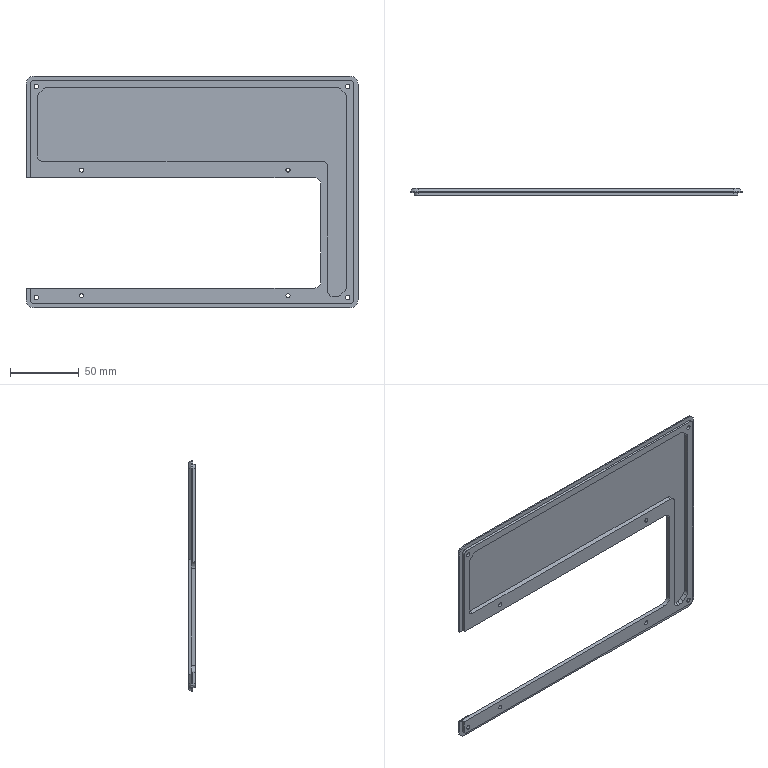CAM job | NX | 3-axis milling, drilling | part box 242 x 5 x 169 mm | stock box 242 x 5 x 169 mm
Tools:
number,name,description,diameter,corner_radius,flute_length,length,flutes
3,T3-D10-CX,Milling Tool-5 Parameters,10.0,0.0,50.0,75.0,2
4,T4-D10-JX,Milling Tool-5 Parameters,10.0,0.0,50.0,75.0,2
10,T10-D4-90度,Drilling Tool,4.0,0.0,35.0,50.0,2
6,T6-D8-JX,Milling Tool-5 Parameters,8.0,0.0,50.0,75.0,2
12,T12-ZT3.2,Drilling Tool,3.2,0.0,35.0,50.0,2
14,T14-ZT2.75,Drilling Tool,2.75,0.0,35.0,50.0,2
15,T15-M3,Drilling Tool,3.0,0.0,35.0,50.0,2
9,T9-D8-90度,Drilling Tool,8.0,0.0,35.0,50.0,2
2,ZT-4.2,Drilling Tool,4.2,0.0,35.0,50.0,2
5,M5,Milling Tool-5 Parameters,5.0,1.0,30.0,30.0,4
Operations:
program,operation,operation_type,tool,method,geometry_group,spindle_rpm,surface_speed,feed_per_tooth,feed_cut,feed_plunge,cut_length_mm,path_length_mm,cut_time_min,machine_time_min
Y01,A1,PlanarMilling,T3-D10-CX,METHOD,WORKPIECE,6500.0,122.0,0.1154,1500.0,100.0,362.0,915.217,0.2413,0.3366
Y01,A2,PlanarMilling,T3-D10-CX,METHOD,WORKPIECE,6500.0,122.0,0.1154,1500.0,100.0,724.0,1659.018,0.4827,0.6536
Y01,A3,PlanarMilling,T4-D10-JX,METHOD,WORKPIECE,6500.0,122.0,0.1154,1500.0,100.0,362.0,915.617,0.2413,0.3367
Y01,A4,PlanarMilling,T4-D10-JX,METHOD,WORKPIECE,6500.0,122.0,0.1154,1500.0,100.0,724.0,1658.618,0.4827,0.6535
Y01,A5,PlanarMilling,T10-D4-90度,METHOD,WORKPIECE,6500.0,81.0,0.0385,500.0,100.0,348.8,890.418,0.6976,0.7907
Y01,A6,PlanarMilling,T10-D4-90度,METHOD,WORKPIECE,6500.0,81.0,0.0385,500.0,100.0,348.8,900.817,0.6976,0.7926
Y02,B1,PlanarMilling,T3-D10-CX,METHOD,WORKPIECE,6500.0,122.0,0.1154,1500.0,100.0,541.681,992.281,0.3611,0.4361
Y02,B2,PlanarMilling,T3-D10-CX,METHOD,WORKPIECE,6500.0,122.0,0.1154,1500.0,100.0,537.398,1007.616,0.3583,0.4366
Y02,B2-1,VolumeBased25DMillingOperation,T3-D10-CX,METHOD,WORKPIECE,6500.0,0.0,0.1538,2000.0,100.0,8660.845,8931.268,12.659,12.695
Y02,B3,PlanarMilling,T4-D10-JX,METHOD,WORKPIECE,6500.0,122.0,0.1154,1500.0,100.0,540.425,991.425,0.3603,0.4353
Y02,B4,PlanarMilling,T4-D10-JX,METHOD,WORKPIECE,6500.0,122.0,0.1154,1500.0,100.0,562.531,1023.748,0.375,0.4516
Y02,B5,VolumeBased25DMillingOperation,T6-D8-JX,METHOD,WORKPIECE,6500.0,163.0,0.1154,1500.0,100.0,3128.304,3328.284,4.214,4.244
Y02,B5_COPY,VolumeBased25DMillingOperation,T6-D8-JX,METHOD,WORKPIECE,6500.0,163.0,0.0769,1000.0,100.0,3129.45,3329.45,5.192,5.222
Y02,B6,PlanarMilling,T10-D4-90度,METHOD,WORKPIECE,6500.0,81.0,0.0385,500.0,100.0,517.292,968.309,1.035,1.11
Y02,B7,PlanarMilling,T10-D4-90度,METHOD,WORKPIECE,6500.0,81.0,0.0385,500.0,100.0,537.398,992.416,1.075,1.15
Y02,B8,PlanarMilling,T10-D4-90度,METHOD,WORKPIECE,6500.0,81.0,0.0385,500.0,100.0,750.9,952.9,1.502,1.532
Y02,B9,Operation,T10-D4-90度,METHOD,WORKPIECE,1200.0,18.0,0.0417,100.0,0.0,12.0,736.517,0.12,0.1925
Y02,B10,Operation,T10-D4-90度,METHOD,WORKPIECE,1200.0,18.0,0.0417,100.0,0.0,12.0,605.653,0.12,0.1794
Y02,B11,Operation,T12-ZT3.2,METHOD,WORKPIECE,1200.0,18.0,0.0417,100.0,0.0,34.0,780.517,0.34,0.4147
Y02,B12,Operation,T14-ZT2.75,METHOD,WORKPIECE,1200.0,18.0,0.0417,100.0,0.0,42.0,665.653,0.42,0.4824
Y02,B13,Operation,T15-M3,METHOD,WORKPIECE,400.0,3.0,0.25,200.0,0.0,34.0,649.653,0.17,0.2316
Y16,C1,PlanarMilling,T3-D10-CX,METHOD,WORKPIECE_1,6500.0,122.0,0.1154,1500.0,100.0,1118.888,1322.688,0.7459,0.7765
Y16,C2,PlanarMilling,T6-D8-JX,METHOD,WORKPIECE_1,6500.0,122.0,0.1154,1500.0,100.0,1127.929,1331.929,0.752,0.7826
Y16,DRILLING_COPY_3,Operation,T9-D8-90度,METHOD,WORKPIECE_1,2000.0,50.0,0.025,100.0,0.0,17.6,468.909,0.176,0.2211
Y16,C3-M00,PlanarMilling,T3-D10-CX,METHOD,WORKPIECE_1,6500.0,122.0,0.1154,1500.0,100.0,511.022,720.422,0.3407,0.3721
Y19,C4,PlanarMilling,T4-D10-JX,METHOD,WORKPIECE_1,6500.0,122.0,0.1154,1500.0,100.0,511.822,722.822,0.3412,0.3729
Y19,C5,PlanarMilling,T10-D4-90度,METHOD,WORKPIECE_1,6500.0,81.0,0.0385,500.0,100.0,538.558,740.558,1.077,1.107
Y19,C6--M00,PlanarMilling,T10-D4-90度,METHOD,WORKPIECE_1,6500.0,81.0,0.0385,500.0,100.0,508.366,714.366,1.017,1.048
Y22,C7,ZLevelMilling,T9-D8-90度,METHOD,WORKPIECE_1,6500.0,163.0,0.0385,500.0,100.0,757.957,963.609,1.516,1.547
工装孔,DRILLING,Operation,T9-D8-90度,METHOD,MCS_MILL,2000.0,50.0,0.025,100.0,0.0,56.0,912.16,0.56,0.6456
工装孔,PLANAR_MILL,PlanarMilling,T9-D8-90度,METHOD,MCS_MILL,5000.0,125.0,0.1,1000.0,100.0,1730.0,1924.0,1.73,1.749
工装孔,DRILLING_COPY,Operation,ZT-4.2,METHOD,MCS_MILL,2000.0,50.0,0.025,100.0,0.0,66.0,341.84,0.66,0.6876
工装孔,DRILLING_COPY_1,Operation,M5,METHOD,MCS_MILL,400.0,6.0,0.2,320.0,0.0,40.0,289.84,0.125,0.15
3.NC,DRILLING_COPY_2,Operation,T9-D8-90度,METHOD,MCS,2000.0,50.0,0.025,100.0,0.0,11.2,169.044,0.112,0.1278
3.NC,DRILLING_COPY_COPY,Operation,ZT-4.2,METHOD,MCS,2000.0,50.0,0.025,100.0,0.0,66.0,278.644,0.66,0.6813
3.NC,DRILLING_COPY_1_COPY,Operation,M5,METHOD,MCS,400.0,6.0,0.2,320.0,0.0,40.0,226.644,0.125,0.1437